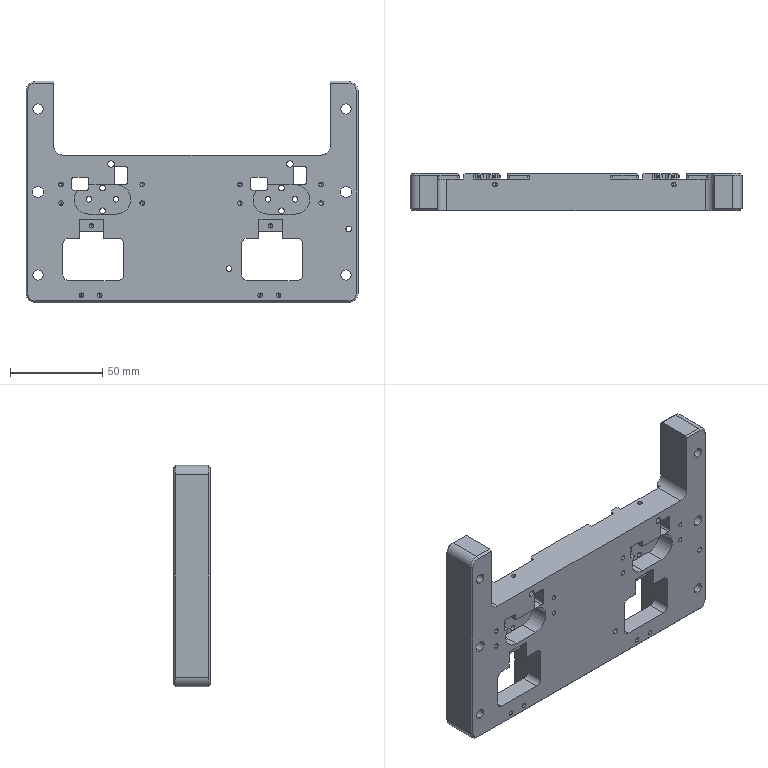Part | STEP file | 07-01 runout inspection base die | 1 solid | 574 faces | box 180 x 20 x 120 mm | volume 238820 mm3 | cylinder 265 | plane 238 | cone 71 | commonest cylinder face diameters 2.5 x56 2 x55 3 x42 1.1 x32 1 x24 10 x14